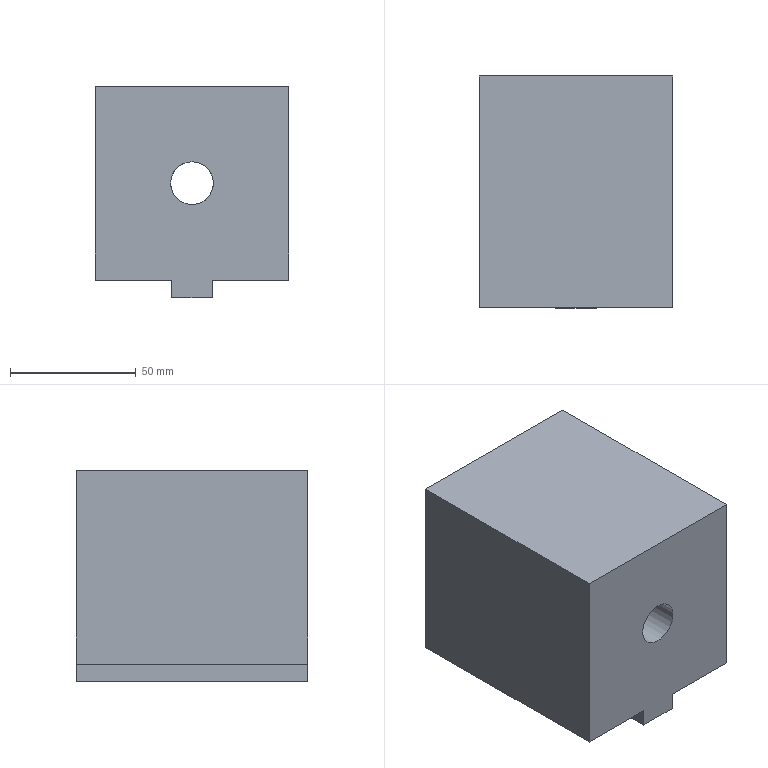Part | NX | features MAIN_BODY 2 | 1 solid | 11 faces | box 77 x 92 x 84 mm | volume 534890 mm3 | plane 10 | cylinder 1 | commonest cylinder face diameters 17 x1
STEP:
#1=CARTESIAN_POINT('',(-335.,38.5,397.5));
#2=VERTEX_POINT('',#1);
#3=CARTESIAN_POINT('',(-335.,38.5,320.5));
#4=VERTEX_POINT('',#3);
#5=CARTESIAN_POINT('',(-335.,38.5,379.));
#6=DIRECTION('',(0.000000001,-0.00000017,-1.));
#7=VECTOR('',#6,1000.);
#8=LINE('',#5,#7);
#9=EDGE_CURVE('',#2,#4,#8,.T.);
#10=ORIENTED_EDGE('',*,*,#9,.T.);
#11=CARTESIAN_POINT('',(-335.,-53.5,320.5));
#12=VERTEX_POINT('',#11);
#13=CARTESIAN_POINT('',(-335.,-53.5,320.5));
#14=DIRECTION('',(-0.000000011,1.,-0.00000017));
#15=VECTOR('',#14,1000.);
#16=LINE('',#13,#15);
#17=EDGE_CURVE('',#12,#4,#16,.T.);
#18=ORIENTED_EDGE('',*,*,#17,.F.);
#19=CARTESIAN_POINT('',(-335.,-53.5,397.5));
#20=VERTEX_POINT('',#19);
#21=CARTESIAN_POINT('',(-335.,-53.5,379.));
#22=DIRECTION('',(0.000000001,-0.00000017,-1.));
#23=VECTOR('',#22,1000.);
#24=LINE('',#21,#23);
#25=EDGE_CURVE('',#20,#12,#24,.T.);
#26=ORIENTED_EDGE('',*,*,#25,.F.);
#27=CARTESIAN_POINT('',(-335.,-53.5,397.5));
#28=DIRECTION('',(-0.000000011,1.,-0.00000017));
#29=VECTOR('',#28,1000.);
#30=LINE('',#27,#29);
#31=EDGE_CURVE('',#20,#2,#30,.T.);
#32=ORIENTED_EDGE('',*,*,#31,.T.);
#33=EDGE_LOOP('',(#10,#18,#26,#32));
#34=FACE_BOUND('',#33,.T.);
#35=CARTESIAN_POINT('',(-335.,-53.5,379.));
#36=DIRECTION('',(-1.,-0.000000011,-0.000000001));
#37=DIRECTION('',(0.000000001,-0.00000017,-1.));
#38=AXIS2_PLACEMENT_3D('',#35,#36,#37);
#39=PLANE('',#38);
#40=ADVANCED_FACE('',(#34),#39,.T.);
#41=CARTESIAN_POINT('',(-304.5,38.5,320.5));
#42=VERTEX_POINT('',#41);
#43=CARTESIAN_POINT('',(-258.,38.5,320.5));
#44=DIRECTION('',(1.,0.000000011,0.000000001));
#45=VECTOR('',#44,1000.);
#46=LINE('',#43,#45);
#47=EDGE_CURVE('',#4,#42,#46,.T.);
#48=ORIENTED_EDGE('',*,*,#47,.T.);
#49=CARTESIAN_POINT('',(-304.5,-53.5,320.5));
#50=VERTEX_POINT('',#49);
#51=CARTESIAN_POINT('',(-304.5,-53.5,320.5));
#52=DIRECTION('',(-0.000000011,1.,-0.00000017));
#53=VECTOR('',#52,1000.);
#54=LINE('',#51,#53);
#55=EDGE_CURVE('',#50,#42,#54,.T.);
#56=ORIENTED_EDGE('',*,*,#55,.F.);
#57=CARTESIAN_POINT('',(-335.,-53.5,320.5));
#58=DIRECTION('',(1.,0.000000011,0.000000001));
#59=VECTOR('',#58,1000.);
#60=LINE('',#57,#59);
#61=EDGE_CURVE('',#12,#50,#60,.T.);
#62=ORIENTED_EDGE('',*,*,#61,.F.);
#63=ORIENTED_EDGE('',*,*,#17,.T.);
#64=EDGE_LOOP('',(#48,#56,#62,#63));
#65=FACE_BOUND('',#64,.T.);
#66=CARTESIAN_POINT('',(-335.,-53.5,320.5));
#67=DIRECTION('',(0.000000001,-0.00000017,-1.));
#68=DIRECTION('',(1.,0.000000011,0.000000001));
#69=AXIS2_PLACEMENT_3D('',#66,#67,#68);
#70=PLANE('',#69);
#71=ADVANCED_FACE('',(#65),#70,.T.);
#72=CARTESIAN_POINT('',(-304.5,38.5,313.5));
#73=VERTEX_POINT('',#72);
#74=CARTESIAN_POINT('',(-304.5,38.5,379.));
#75=DIRECTION('',(0.000000001,-0.00000017,-1.));
#76=VECTOR('',#75,1000.);
#77=LINE('',#74,#76);
#78=EDGE_CURVE('',#42,#73,#77,.T.);
#79=ORIENTED_EDGE('',*,*,#78,.T.);
#80=CARTESIAN_POINT('',(-304.5,-53.5,313.5));
#81=VERTEX_POINT('',#80);
#82=CARTESIAN_POINT('',(-304.5,-53.5,313.5));
#83=DIRECTION('',(-0.000000011,1.,-0.00000017));
#84=VECTOR('',#83,1000.);
#85=LINE('',#82,#84);
#86=EDGE_CURVE('',#81,#73,#85,.T.);
#87=ORIENTED_EDGE('',*,*,#86,.F.);
#88=CARTESIAN_POINT('',(-304.5,-53.5,320.5));
#89=DIRECTION('',(0.000000001,-0.00000017,-1.));
#90=VECTOR('',#89,1000.);
#91=LINE('',#88,#90);
#92=EDGE_CURVE('',#50,#81,#91,.T.);
#93=ORIENTED_EDGE('',*,*,#92,.F.);
#94=ORIENTED_EDGE('',*,*,#55,.T.);
#95=EDGE_LOOP('',(#79,#87,#93,#94));
#96=FACE_BOUND('',#95,.T.);
#97=CARTESIAN_POINT('',(-304.5,-53.5,320.5));
#98=DIRECTION('',(-1.,-0.000000011,-0.000000001));
#99=DIRECTION('',(0.000000001,-0.00000017,-1.));
#100=AXIS2_PLACEMENT_3D('',#97,#98,#99);
#101=PLANE('',#100);
#102=ADVANCED_FACE('',(#96),#101,.T.);
#103=CARTESIAN_POINT('',(-288.5,38.5,313.5));
#104=VERTEX_POINT('',#103);
#105=CARTESIAN_POINT('',(-258.,38.5,313.5));
#106=DIRECTION('',(1.,0.000000011,0.000000001));
#107=VECTOR('',#106,1000.);
#108=LINE('',#105,#107);
#109=EDGE_CURVE('',#73,#104,#108,.T.);
#110=ORIENTED_EDGE('',*,*,#109,.T.);
#111=CARTESIAN_POINT('',(-288.5,-53.5,313.5));
#112=VERTEX_POINT('',#111);
#113=CARTESIAN_POINT('',(-288.5,-53.5,313.5));
#114=DIRECTION('',(-0.000000011,1.,-0.00000017));
#115=VECTOR('',#114,1000.);
#116=LINE('',#113,#115);
#117=EDGE_CURVE('',#112,#104,#116,.T.);
#118=ORIENTED_EDGE('',*,*,#117,.F.);
#119=CARTESIAN_POINT('',(-304.5,-53.5,313.5));
#120=DIRECTION('',(1.,0.000000011,0.000000001));
#121=VECTOR('',#120,1000.);
#122=LINE('',#119,#121);
#123=EDGE_CURVE('',#81,#112,#122,.T.);
#124=ORIENTED_EDGE('',*,*,#123,.F.);
#125=ORIENTED_EDGE('',*,*,#86,.T.);
#126=EDGE_LOOP('',(#110,#118,#124,#125));
#127=FACE_BOUND('',#126,.T.);
#128=CARTESIAN_POINT('',(-304.5,-53.5,313.5));
#129=DIRECTION('',(0.000000001,-0.00000017,-1.));
#130=DIRECTION('',(1.,0.000000011,0.000000001));
#131=AXIS2_PLACEMENT_3D('',#128,#129,#130);
#132=PLANE('',#131);
#133=ADVANCED_FACE('',(#127),#132,.T.);
#134=CARTESIAN_POINT('',(-288.5,38.5,320.5));
#135=VERTEX_POINT('',#134);
#136=CARTESIAN_POINT('',(-288.5,38.5,379.));
#137=DIRECTION('',(-0.000000001,0.00000017,1.));
#138=VECTOR('',#137,1000.);
#139=LINE('',#136,#138);
#140=EDGE_CURVE('',#104,#135,#139,.T.);
#141=ORIENTED_EDGE('',*,*,#140,.T.);
#142=CARTESIAN_POINT('',(-288.5,-53.5,320.5));
#143=VERTEX_POINT('',#142);
#144=CARTESIAN_POINT('',(-288.5,-53.5,320.5));
#145=DIRECTION('',(-0.000000011,1.,-0.00000017));
#146=VECTOR('',#145,1000.);
#147=LINE('',#144,#146);
#148=EDGE_CURVE('',#143,#135,#147,.T.);
#149=ORIENTED_EDGE('',*,*,#148,.F.);
#150=CARTESIAN_POINT('',(-288.5,-53.5,313.5));
#151=DIRECTION('',(-0.000000001,0.00000017,1.));
#152=VECTOR('',#151,1000.);
#153=LINE('',#150,#152);
#154=EDGE_CURVE('',#112,#143,#153,.T.);
#155=ORIENTED_EDGE('',*,*,#154,.F.);
#156=ORIENTED_EDGE('',*,*,#117,.T.);
#157=EDGE_LOOP('',(#141,#149,#155,#156));
#158=FACE_BOUND('',#157,.T.);
#159=CARTESIAN_POINT('',(-288.5,-53.5,313.5));
#160=DIRECTION('',(1.,0.000000011,0.000000001));
#161=DIRECTION('',(-0.000000001,0.00000017,1.));
#162=AXIS2_PLACEMENT_3D('',#159,#160,#161);
#163=PLANE('',#162);
#164=ADVANCED_FACE('',(#158),#163,.T.);
#165=CARTESIAN_POINT('',(-258.,38.5,320.5));
#166=VERTEX_POINT('',#165);
#167=CARTESIAN_POINT('',(-258.,38.5,320.5));
#168=DIRECTION('',(1.,0.000000011,0.000000001));
#169=VECTOR('',#168,1000.);
#170=LINE('',#167,#169);
#171=EDGE_CURVE('',#135,#166,#170,.T.);
#172=ORIENTED_EDGE('',*,*,#171,.T.);
#173=CARTESIAN_POINT('',(-258.,-53.5,320.5));
#174=VERTEX_POINT('',#173);
#175=CARTESIAN_POINT('',(-258.,-53.5,320.5));
#176=DIRECTION('',(-0.000000011,1.,-0.00000017));
#177=VECTOR('',#176,1000.);
#178=LINE('',#175,#177);
#179=EDGE_CURVE('',#174,#166,#178,.T.);
#180=ORIENTED_EDGE('',*,*,#179,.F.);
#181=CARTESIAN_POINT('',(-288.5,-53.5,320.5));
#182=DIRECTION('',(1.,0.000000011,0.000000001));
#183=VECTOR('',#182,1000.);
#184=LINE('',#181,#183);
#185=EDGE_CURVE('',#143,#174,#184,.T.);
#186=ORIENTED_EDGE('',*,*,#185,.F.);
#187=ORIENTED_EDGE('',*,*,#148,.T.);
#188=EDGE_LOOP('',(#172,#180,#186,#187));
#189=FACE_BOUND('',#188,.T.);
#190=CARTESIAN_POINT('',(-288.5,-53.5,320.5));
#191=DIRECTION('',(0.000000001,-0.00000017,-1.));
#192=DIRECTION('',(1.,0.000000011,0.000000001));
#193=AXIS2_PLACEMENT_3D('',#190,#191,#192);
#194=PLANE('',#193);
#195=ADVANCED_FACE('',(#189),#194,.T.);
#196=CARTESIAN_POINT('',(-258.,38.5,397.5));
#197=VERTEX_POINT('',#196);
#198=CARTESIAN_POINT('',(-258.,38.5,379.));
#199=DIRECTION('',(-0.000000001,0.00000017,1.));
#200=VECTOR('',#199,1000.);
#201=LINE('',#198,#200);
#202=EDGE_CURVE('',#166,#197,#201,.T.);
#203=ORIENTED_EDGE('',*,*,#202,.T.);
#204=CARTESIAN_POINT('',(-258.,-53.5,397.5));
#205=VERTEX_POINT('',#204);
#206=CARTESIAN_POINT('',(-258.,73.5,397.5));
#207=DIRECTION('',(0.000000011,-1.,0.00000017));
#208=VECTOR('',#207,1000.);
#209=LINE('',#206,#208);
#210=EDGE_CURVE('',#197,#205,#209,.T.);
#211=ORIENTED_EDGE('',*,*,#210,.T.);
#212=CARTESIAN_POINT('',(-258.,-53.5,320.5));
#213=DIRECTION('',(-0.000000001,0.00000017,1.));
#214=VECTOR('',#213,1000.);
#215=LINE('',#212,#214);
#216=EDGE_CURVE('',#174,#205,#215,.T.);
#217=ORIENTED_EDGE('',*,*,#216,.F.);
#218=ORIENTED_EDGE('',*,*,#179,.T.);
#219=EDGE_LOOP('',(#203,#211,#217,#218));
#220=FACE_BOUND('',#219,.T.);
#221=CARTESIAN_POINT('',(-258.,-53.5,348.));
#222=DIRECTION('',(1.,0.000000011,0.000000001));
#223=DIRECTION('',(-0.000000001,0.00000017,1.));
#224=AXIS2_PLACEMENT_3D('',#221,#222,#223);
#225=PLANE('',#224);
#226=ADVANCED_FACE('',(#220),#225,.T.);
#227=CARTESIAN_POINT('',(-305.,-53.5,359.));
#228=VERTEX_POINT('',#227);
#229=CARTESIAN_POINT('',(-296.5,-53.5,359.));
#230=DIRECTION('',(0.000000011,-1.,0.00000017));
#231=DIRECTION('',(-1.,-0.000000011,-0.000000001));
#232=AXIS2_PLACEMENT_3D('',#229,#230,#231);
#233=CIRCLE('',#232,8.5);
#234=EDGE_CURVE('',#228,#228,#233,.T.);
#235=ORIENTED_EDGE('',*,*,#234,.F.);
#236=EDGE_LOOP('',(#235));
#237=FACE_BOUND('',#236,.T.);
#238=CARTESIAN_POINT('',(-258.,-53.5,397.5));
#239=DIRECTION('',(-1.,-0.000000011,-0.000000001));
#240=VECTOR('',#239,1000.);
#241=LINE('',#238,#240);
#242=EDGE_CURVE('',#205,#20,#241,.T.);
#243=ORIENTED_EDGE('',*,*,#242,.T.);
#244=ORIENTED_EDGE('',*,*,#25,.T.);
#245=ORIENTED_EDGE('',*,*,#61,.T.);
#246=ORIENTED_EDGE('',*,*,#92,.T.);
#247=ORIENTED_EDGE('',*,*,#123,.T.);
#248=ORIENTED_EDGE('',*,*,#154,.T.);
#249=ORIENTED_EDGE('',*,*,#185,.T.);
#250=ORIENTED_EDGE('',*,*,#216,.T.);
#251=EDGE_LOOP('',(#243,#244,#245,#246,#247,#248,#249,#250));
#252=FACE_BOUND('',#251,.T.);
#253=CARTESIAN_POINT('',(-258.,-53.5,379.));
#254=DIRECTION('',(-0.000000011,1.,-0.00000017));
#255=DIRECTION('',(-0.000000001,0.00000017,1.));
#256=AXIS2_PLACEMENT_3D('',#253,#254,#255);
#257=PLANE('',#256);
#258=ADVANCED_FACE('',(#237,#252),#257,.F.);
#259=CARTESIAN_POINT('',(-296.5,38.5,367.5));
#260=VERTEX_POINT('',#259);
#261=CARTESIAN_POINT('',(-296.5,38.5,359.));
#262=DIRECTION('',(0.000000011,-1.,0.00000017));
#263=DIRECTION('',(-0.000000001,0.00000017,1.));
#264=AXIS2_PLACEMENT_3D('',#261,#262,#263);
#265=CIRCLE('',#264,8.5);
#266=EDGE_CURVE('',#260,#260,#265,.T.);
#267=ORIENTED_EDGE('',*,*,#266,.T.);
#268=EDGE_LOOP('',(#267));
#269=FACE_BOUND('',#268,.T.);
#270=ORIENTED_EDGE('',*,*,#202,.F.);
#271=ORIENTED_EDGE('',*,*,#171,.F.);
#272=ORIENTED_EDGE('',*,*,#140,.F.);
#273=ORIENTED_EDGE('',*,*,#109,.F.);
#274=ORIENTED_EDGE('',*,*,#78,.F.);
#275=ORIENTED_EDGE('',*,*,#47,.F.);
#276=ORIENTED_EDGE('',*,*,#9,.F.);
#277=CARTESIAN_POINT('',(-335.,38.5,397.5));
#278=DIRECTION('',(1.,0.000000011,0.000000001));
#279=VECTOR('',#278,1000.);
#280=LINE('',#277,#279);
#281=EDGE_CURVE('',#2,#197,#280,.T.);
#282=ORIENTED_EDGE('',*,*,#281,.T.);
#283=EDGE_LOOP('',(#270,#271,#272,#273,#274,#275,#276,#282));
#284=FACE_BOUND('',#283,.T.);
#285=CARTESIAN_POINT('',(-258.,38.5,379.));
#286=DIRECTION('',(-0.000000011,1.,-0.00000017));
#287=DIRECTION('',(-0.000000001,0.00000017,1.));
#288=AXIS2_PLACEMENT_3D('',#285,#286,#287);
#289=PLANE('',#288);
#290=ADVANCED_FACE('',(#269,#284),#289,.T.);
#291=ORIENTED_EDGE('',*,*,#234,.T.);
#292=EDGE_LOOP('',(#291));
#293=FACE_BOUND('',#292,.T.);
#294=ORIENTED_EDGE('',*,*,#266,.F.);
#295=EDGE_LOOP('',(#294));
#296=FACE_BOUND('',#295,.T.);
#297=CARTESIAN_POINT('',(-296.5,-53.5,359.));
#298=DIRECTION('',(-0.000000011,1.,-0.00000017));
#299=DIRECTION('',(-0.000000001,0.00000017,1.));
#300=AXIS2_PLACEMENT_3D('',#297,#298,#299);
#301=CYLINDRICAL_SURFACE('',#300,8.5);
#302=ADVANCED_FACE('',(#293,#296),#301,.F.);
#303=ORIENTED_EDGE('',*,*,#242,.F.);
#304=ORIENTED_EDGE('',*,*,#210,.F.);
#305=ORIENTED_EDGE('',*,*,#281,.F.);
#306=ORIENTED_EDGE('',*,*,#31,.F.);
#307=EDGE_LOOP('',(#303,#304,#305,#306));
#308=FACE_BOUND('',#307,.T.);
#309=CARTESIAN_POINT('',(-335.,-53.5,397.5));
#310=DIRECTION('',(-0.000000001,0.00000017,1.));
#311=DIRECTION('',(-1.,-0.000000011,-0.000000001));
#312=AXIS2_PLACEMENT_3D('',#309,#310,#311);
#313=PLANE('',#312);
#314=ADVANCED_FACE('',(#308),#313,.T.);
#315=CLOSED_SHELL('',(#40,#71,#102,#133,#164,#195,#226,#258,#290,#302,#314));
#316=MANIFOLD_SOLID_BREP('',#315);
#317=(LENGTH_UNIT()NAMED_UNIT(*)SI_UNIT(.MILLI.,.METRE.));
#318=UNCERTAINTY_MEASURE_WITH_UNIT(LENGTH_MEASURE(0.00001),#317,'','');
#319=(NAMED_UNIT(*)PLANE_ANGLE_UNIT()SI_UNIT($,.RADIAN.));
#320=(NAMED_UNIT(*)SI_UNIT($,.STERADIAN.)SOLID_ANGLE_UNIT());
#321=(GEOMETRIC_REPRESENTATION_CONTEXT(3)GLOBAL_UNCERTAINTY_ASSIGNED_CONTEXT((#318))GLOBAL_UNIT_ASSIGNED_CONTEXT((#317,#319,#320))REPRESENTATION_CONTEXT('',''));
#322=ADVANCED_BREP_SHAPE_REPRESENTATION('',(#316),#321);